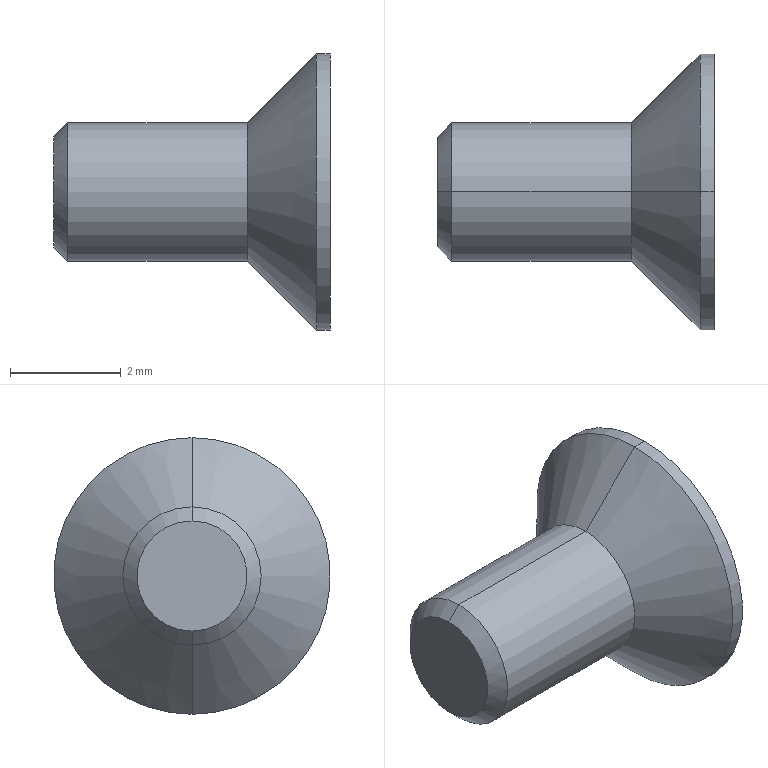Part | STEP file | 1 solid | 17 faces | box 5 x 5 x 5 mm | volume 34.882 mm3 | plane 9 | cylinder 4 | cone 4 | commonest cylinder face diameters 2.5 x2 5 x2
STEP:
#1=CARTESIAN_POINT('',(19.05,-14.605,5.12));
#2=VERTEX_POINT('',#1);
#3=CARTESIAN_POINT('',(19.05,-14.605,10.12));
#4=VERTEX_POINT('',#3);
#5=CARTESIAN_POINT('',(19.05,-14.605,7.62));
#6=DIRECTION('',(1.,0.,0.));
#7=DIRECTION('',(0.,0.,1.));
#8=AXIS2_PLACEMENT_3D('',#5,#6,#7);
#9=CIRCLE('',#8,2.5);
#10=EDGE_CURVE('',#2,#4,#9,.T.);
#11=ORIENTED_EDGE('',*,*,#10,.F.);
#12=CARTESIAN_POINT('',(18.8,-14.605,5.12));
#13=VERTEX_POINT('',#12);
#14=CARTESIAN_POINT('',(19.05,-14.605,5.12));
#15=DIRECTION('',(-1.,0.,0.));
#16=VECTOR('',#15,1000.);
#17=LINE('',#14,#16);
#18=EDGE_CURVE('',#2,#13,#17,.T.);
#19=ORIENTED_EDGE('',*,*,#18,.T.);
#20=CARTESIAN_POINT('',(18.8,-14.605,10.12));
#21=VERTEX_POINT('',#20);
#22=CARTESIAN_POINT('',(18.8,-14.605,7.62));
#23=DIRECTION('',(1.,0.,0.));
#24=DIRECTION('',(0.,0.,1.));
#25=AXIS2_PLACEMENT_3D('',#22,#23,#24);
#26=CIRCLE('',#25,2.5);
#27=EDGE_CURVE('',#13,#21,#26,.T.);
#28=ORIENTED_EDGE('',*,*,#27,.T.);
#29=CARTESIAN_POINT('',(19.05,-14.605,10.12));
#30=DIRECTION('',(-1.,0.,0.));
#31=VECTOR('',#30,1000.);
#32=LINE('',#29,#31);
#33=EDGE_CURVE('',#4,#21,#32,.T.);
#34=ORIENTED_EDGE('',*,*,#33,.F.);
#35=EDGE_LOOP('',(#11,#19,#28,#34));
#36=FACE_OUTER_BOUND('',#35,.T.);
#37=CARTESIAN_POINT('',(19.05,-14.605,7.62));
#38=DIRECTION('',(-1.,0.,0.));
#39=DIRECTION('',(0.,0.,1.));
#40=AXIS2_PLACEMENT_3D('',#37,#38,#39);
#41=CYLINDRICAL_SURFACE('',#40,2.5);
#42=ADVANCED_FACE('',(#36),#41,.T.);
#43=CARTESIAN_POINT('',(17.55,-14.605,6.37));
#44=VERTEX_POINT('',#43);
#45=CARTESIAN_POINT('',(17.55,-14.605,8.87));
#46=VERTEX_POINT('',#45);
#47=CARTESIAN_POINT('',(17.55,-14.605,7.62));
#48=DIRECTION('',(1.,0.,0.));
#49=DIRECTION('',(0.,0.,-1.));
#50=AXIS2_PLACEMENT_3D('',#47,#48,#49);
#51=CIRCLE('',#50,1.25);
#52=EDGE_CURVE('',#44,#46,#51,.T.);
#53=ORIENTED_EDGE('',*,*,#52,.T.);
#54=CARTESIAN_POINT('',(18.8,-14.605,10.12));
#55=DIRECTION('',(0.7071,0.,0.7071));
#56=VECTOR('',#55,1000.);
#57=LINE('',#54,#56);
#58=EDGE_CURVE('',#46,#21,#57,.T.);
#59=ORIENTED_EDGE('',*,*,#58,.T.);
#60=ORIENTED_EDGE('',*,*,#27,.F.);
#61=CARTESIAN_POINT('',(18.8,-14.605,5.12));
#62=DIRECTION('',(0.7071,0.,-0.7071));
#63=VECTOR('',#62,1000.);
#64=LINE('',#61,#63);
#65=EDGE_CURVE('',#44,#13,#64,.T.);
#66=ORIENTED_EDGE('',*,*,#65,.F.);
#67=EDGE_LOOP('',(#53,#59,#60,#66));
#68=FACE_OUTER_BOUND('',#67,.T.);
#69=CARTESIAN_POINT('',(18.8,-14.605,7.62));
#70=DIRECTION('',(1.,0.,0.));
#71=DIRECTION('',(0.,0.,-1.));
#72=AXIS2_PLACEMENT_3D('',#69,#70,#71);
#73=CONICAL_SURFACE('',#72,2.5,0.7854);
#74=ADVANCED_FACE('',(#68),#73,.T.);
#75=ORIENTED_EDGE('',*,*,#52,.F.);
#76=CARTESIAN_POINT('',(14.304,-14.605,6.37));
#77=VERTEX_POINT('',#76);
#78=CARTESIAN_POINT('',(19.05,-14.605,6.37));
#79=DIRECTION('',(-1.,0.,0.));
#80=VECTOR('',#79,1000.);
#81=LINE('',#78,#80);
#82=EDGE_CURVE('',#44,#77,#81,.T.);
#83=ORIENTED_EDGE('',*,*,#82,.T.);
#84=CARTESIAN_POINT('',(14.304,-14.605,8.87));
#85=VERTEX_POINT('',#84);
#86=CARTESIAN_POINT('',(14.304,-14.605,7.62));
#87=DIRECTION('',(1.,0.,0.));
#88=DIRECTION('',(0.,0.,1.));
#89=AXIS2_PLACEMENT_3D('',#86,#87,#88);
#90=CIRCLE('',#89,1.25);
#91=EDGE_CURVE('',#77,#85,#90,.T.);
#92=ORIENTED_EDGE('',*,*,#91,.T.);
#93=CARTESIAN_POINT('',(19.05,-14.605,8.87));
#94=DIRECTION('',(-1.,0.,0.));
#95=VECTOR('',#94,1000.);
#96=LINE('',#93,#95);
#97=EDGE_CURVE('',#46,#85,#96,.T.);
#98=ORIENTED_EDGE('',*,*,#97,.F.);
#99=EDGE_LOOP('',(#75,#83,#92,#98));
#100=FACE_OUTER_BOUND('',#99,.T.);
#101=CARTESIAN_POINT('',(19.05,-14.605,7.62));
#102=DIRECTION('',(-1.,0.,0.));
#103=DIRECTION('',(0.,0.,1.));
#104=AXIS2_PLACEMENT_3D('',#101,#102,#103);
#105=CYLINDRICAL_SURFACE('',#104,1.25);
#106=ADVANCED_FACE('',(#100),#105,.T.);
#107=CARTESIAN_POINT('',(14.05,-14.605,6.624));
#108=VERTEX_POINT('',#107);
#109=CARTESIAN_POINT('',(14.05,-14.605,8.616));
#110=VERTEX_POINT('',#109);
#111=CARTESIAN_POINT('',(14.05,-14.605,7.62));
#112=DIRECTION('',(1.,0.,0.));
#113=DIRECTION('',(0.,0.,-1.));
#114=AXIS2_PLACEMENT_3D('',#111,#112,#113);
#115=CIRCLE('',#114,0.996);
#116=EDGE_CURVE('',#108,#110,#115,.T.);
#117=ORIENTED_EDGE('',*,*,#116,.T.);
#118=CARTESIAN_POINT('',(14.304,-14.605,8.87));
#119=DIRECTION('',(0.7071,0.,0.7071));
#120=VECTOR('',#119,1000.);
#121=LINE('',#118,#120);
#122=EDGE_CURVE('',#110,#85,#121,.T.);
#123=ORIENTED_EDGE('',*,*,#122,.T.);
#124=ORIENTED_EDGE('',*,*,#91,.F.);
#125=CARTESIAN_POINT('',(14.304,-14.605,6.37));
#126=DIRECTION('',(0.7071,0.,-0.7071));
#127=VECTOR('',#126,1000.);
#128=LINE('',#125,#127);
#129=EDGE_CURVE('',#108,#77,#128,.T.);
#130=ORIENTED_EDGE('',*,*,#129,.F.);
#131=EDGE_LOOP('',(#117,#123,#124,#130));
#132=FACE_OUTER_BOUND('',#131,.T.);
#133=CARTESIAN_POINT('',(14.304,-14.605,7.62));
#134=DIRECTION('',(1.,0.,0.));
#135=DIRECTION('',(0.,0.,-1.));
#136=AXIS2_PLACEMENT_3D('',#133,#134,#135);
#137=CONICAL_SURFACE('',#136,1.25,0.7854);
#138=ADVANCED_FACE('',(#132),#137,.T.);
#139=CARTESIAN_POINT('',(19.05,-13.907,8.023));
#140=VERTEX_POINT('',#139);
#141=CARTESIAN_POINT('',(19.05,-13.907,7.217));
#142=VERTEX_POINT('',#141);
#143=CARTESIAN_POINT('',(19.05,-13.907,7.62));
#144=DIRECTION('',(0.,0.,-1.));
#145=VECTOR('',#144,1000.);
#146=LINE('',#143,#145);
#147=EDGE_CURVE('',#140,#142,#146,.T.);
#148=ORIENTED_EDGE('',*,*,#147,.T.);
#149=CARTESIAN_POINT('',(19.05,-14.605,6.813));
#150=VERTEX_POINT('',#149);
#151=CARTESIAN_POINT('',(19.05,-13.907,7.217));
#152=DIRECTION('',(0.,-0.866,-0.5));
#153=VECTOR('',#152,1000.);
#154=LINE('',#151,#153);
#155=EDGE_CURVE('',#142,#150,#154,.T.);
#156=ORIENTED_EDGE('',*,*,#155,.T.);
#157=CARTESIAN_POINT('',(19.05,-15.303,7.217));
#158=VERTEX_POINT('',#157);
#159=CARTESIAN_POINT('',(19.05,-14.605,6.813));
#160=DIRECTION('',(0.,-0.866,0.5));
#161=VECTOR('',#160,1000.);
#162=LINE('',#159,#161);
#163=EDGE_CURVE('',#150,#158,#162,.T.);
#164=ORIENTED_EDGE('',*,*,#163,.T.);
#165=CARTESIAN_POINT('',(19.05,-15.303,8.023));
#166=VERTEX_POINT('',#165);
#167=CARTESIAN_POINT('',(19.05,-15.303,7.62));
#168=DIRECTION('',(0.,0.,1.));
#169=VECTOR('',#168,1000.);
#170=LINE('',#167,#169);
#171=EDGE_CURVE('',#158,#166,#170,.T.);
#172=ORIENTED_EDGE('',*,*,#171,.T.);
#173=CARTESIAN_POINT('',(19.05,-14.605,8.427));
#174=VERTEX_POINT('',#173);
#175=CARTESIAN_POINT('',(19.05,-15.303,8.023));
#176=DIRECTION('',(0.,0.866,0.5));
#177=VECTOR('',#176,1000.);
#178=LINE('',#175,#177);
#179=EDGE_CURVE('',#166,#174,#178,.T.);
#180=ORIENTED_EDGE('',*,*,#179,.T.);
#181=CARTESIAN_POINT('',(19.05,-14.605,8.427));
#182=DIRECTION('',(0.,0.866,-0.5));
#183=VECTOR('',#182,1000.);
#184=LINE('',#181,#183);
#185=EDGE_CURVE('',#174,#140,#184,.T.);
#186=ORIENTED_EDGE('',*,*,#185,.T.);
#187=EDGE_LOOP('',(#148,#156,#164,#172,#180,#186));
#188=FACE_BOUND('',#187,.T.);
#189=CARTESIAN_POINT('',(19.05,-14.605,7.62));
#190=DIRECTION('',(1.,0.,0.));
#191=DIRECTION('',(0.,0.,1.));
#192=AXIS2_PLACEMENT_3D('',#189,#190,#191);
#193=CIRCLE('',#192,2.5);
#194=EDGE_CURVE('',#4,#2,#193,.T.);
#195=ORIENTED_EDGE('',*,*,#194,.T.);
#196=ORIENTED_EDGE('',*,*,#10,.T.);
#197=EDGE_LOOP('',(#195,#196));
#198=FACE_OUTER_BOUND('',#197,.T.);
#199=CARTESIAN_POINT('',(19.05,-12.105,7.62));
#200=DIRECTION('',(1.,0.,0.));
#201=DIRECTION('',(0.,1.,0.));
#202=AXIS2_PLACEMENT_3D('',#199,#200,#201);
#203=PLANE('',#202);
#204=ADVANCED_FACE('',(#188,#198),#203,.T.);
#205=ORIENTED_EDGE('',*,*,#18,.F.);
#206=ORIENTED_EDGE('',*,*,#194,.F.);
#207=ORIENTED_EDGE('',*,*,#33,.T.);
#208=CARTESIAN_POINT('',(18.8,-14.605,7.62));
#209=DIRECTION('',(1.,0.,0.));
#210=DIRECTION('',(0.,0.,1.));
#211=AXIS2_PLACEMENT_3D('',#208,#209,#210);
#212=CIRCLE('',#211,2.5);
#213=EDGE_CURVE('',#21,#13,#212,.T.);
#214=ORIENTED_EDGE('',*,*,#213,.T.);
#215=EDGE_LOOP('',(#205,#206,#207,#214));
#216=FACE_OUTER_BOUND('',#215,.T.);
#217=CARTESIAN_POINT('',(19.05,-14.605,7.62));
#218=DIRECTION('',(-1.,0.,0.));
#219=DIRECTION('',(0.,0.,1.));
#220=AXIS2_PLACEMENT_3D('',#217,#218,#219);
#221=CYLINDRICAL_SURFACE('',#220,2.5);
#222=ADVANCED_FACE('',(#216),#221,.T.);
#223=CARTESIAN_POINT('',(18.288,-13.907,7.217));
#224=VERTEX_POINT('',#223);
#225=CARTESIAN_POINT('',(18.288,-13.907,7.217));
#226=DIRECTION('',(1.,0.,0.));
#227=VECTOR('',#226,1000.);
#228=LINE('',#225,#227);
#229=EDGE_CURVE('',#224,#142,#228,.T.);
#230=ORIENTED_EDGE('',*,*,#229,.F.);
#231=CARTESIAN_POINT('',(18.288,-14.605,6.813));
#232=VERTEX_POINT('',#231);
#233=CARTESIAN_POINT('',(18.288,-14.605,6.813));
#234=DIRECTION('',(0.,0.866,0.5));
#235=VECTOR('',#234,1000.);
#236=LINE('',#233,#235);
#237=EDGE_CURVE('',#232,#224,#236,.T.);
#238=ORIENTED_EDGE('',*,*,#237,.F.);
#239=CARTESIAN_POINT('',(18.288,-14.605,6.813));
#240=DIRECTION('',(-1.,0.,0.));
#241=VECTOR('',#240,1000.);
#242=LINE('',#239,#241);
#243=EDGE_CURVE('',#150,#232,#242,.T.);
#244=ORIENTED_EDGE('',*,*,#243,.F.);
#245=ORIENTED_EDGE('',*,*,#155,.F.);
#246=EDGE_LOOP('',(#230,#238,#244,#245));
#247=FACE_OUTER_BOUND('',#246,.T.);
#248=CARTESIAN_POINT('',(18.288,-14.605,6.813));
#249=DIRECTION('',(0.,0.5,-0.866));
#250=DIRECTION('',(-1.,0.,0.));
#251=AXIS2_PLACEMENT_3D('',#248,#249,#250);
#252=PLANE('',#251);
#253=ADVANCED_FACE('',(#247),#252,.F.);
#254=CARTESIAN_POINT('',(18.288,-13.907,8.023));
#255=VERTEX_POINT('',#254);
#256=CARTESIAN_POINT('',(18.288,-13.907,8.023));
#257=DIRECTION('',(1.,0.,0.));
#258=VECTOR('',#257,1000.);
#259=LINE('',#256,#258);
#260=EDGE_CURVE('',#255,#140,#259,.T.);
#261=ORIENTED_EDGE('',*,*,#260,.F.);
#262=CARTESIAN_POINT('',(18.288,-13.907,7.217));
#263=DIRECTION('',(0.,0.,1.));
#264=VECTOR('',#263,1000.);
#265=LINE('',#262,#264);
#266=EDGE_CURVE('',#224,#255,#265,.T.);
#267=ORIENTED_EDGE('',*,*,#266,.F.);
#268=ORIENTED_EDGE('',*,*,#229,.T.);
#269=ORIENTED_EDGE('',*,*,#147,.F.);
#270=EDGE_LOOP('',(#261,#267,#268,#269));
#271=FACE_OUTER_BOUND('',#270,.T.);
#272=CARTESIAN_POINT('',(18.288,-13.907,7.217));
#273=DIRECTION('',(0.,1.,0.));
#274=DIRECTION('',(0.,0.,-1.));
#275=AXIS2_PLACEMENT_3D('',#272,#273,#274);
#276=PLANE('',#275);
#277=ADVANCED_FACE('',(#271),#276,.F.);
#278=CARTESIAN_POINT('',(18.288,-14.605,8.427));
#279=VERTEX_POINT('',#278);
#280=CARTESIAN_POINT('',(18.288,-14.605,8.427));
#281=DIRECTION('',(1.,0.,0.));
#282=VECTOR('',#281,1000.);
#283=LINE('',#280,#282);
#284=EDGE_CURVE('',#279,#174,#283,.T.);
#285=ORIENTED_EDGE('',*,*,#284,.F.);
#286=CARTESIAN_POINT('',(18.288,-13.907,8.023));
#287=DIRECTION('',(0.,-0.866,0.5));
#288=VECTOR('',#287,1000.);
#289=LINE('',#286,#288);
#290=EDGE_CURVE('',#255,#279,#289,.T.);
#291=ORIENTED_EDGE('',*,*,#290,.F.);
#292=ORIENTED_EDGE('',*,*,#260,.T.);
#293=ORIENTED_EDGE('',*,*,#185,.F.);
#294=EDGE_LOOP('',(#285,#291,#292,#293));
#295=FACE_OUTER_BOUND('',#294,.T.);
#296=CARTESIAN_POINT('',(18.288,-13.907,8.023));
#297=DIRECTION('',(0.,0.5,0.866));
#298=DIRECTION('',(1.,0.,0.));
#299=AXIS2_PLACEMENT_3D('',#296,#297,#298);
#300=PLANE('',#299);
#301=ADVANCED_FACE('',(#295),#300,.F.);
#302=CARTESIAN_POINT('',(18.288,-15.303,8.023));
#303=VERTEX_POINT('',#302);
#304=CARTESIAN_POINT('',(18.288,-15.303,8.023));
#305=DIRECTION('',(1.,0.,0.));
#306=VECTOR('',#305,1000.);
#307=LINE('',#304,#306);
#308=EDGE_CURVE('',#303,#166,#307,.T.);
#309=ORIENTED_EDGE('',*,*,#308,.F.);
#310=CARTESIAN_POINT('',(18.288,-14.605,8.427));
#311=DIRECTION('',(0.,-0.866,-0.5));
#312=VECTOR('',#311,1000.);
#313=LINE('',#310,#312);
#314=EDGE_CURVE('',#279,#303,#313,.T.);
#315=ORIENTED_EDGE('',*,*,#314,.F.);
#316=ORIENTED_EDGE('',*,*,#284,.T.);
#317=ORIENTED_EDGE('',*,*,#179,.F.);
#318=EDGE_LOOP('',(#309,#315,#316,#317));
#319=FACE_OUTER_BOUND('',#318,.T.);
#320=CARTESIAN_POINT('',(18.288,-14.605,8.427));
#321=DIRECTION('',(0.,-0.5,0.866));
#322=DIRECTION('',(-1.,0.,0.));
#323=AXIS2_PLACEMENT_3D('',#320,#321,#322);
#324=PLANE('',#323);
#325=ADVANCED_FACE('',(#319),#324,.F.);
#326=CARTESIAN_POINT('',(18.288,-15.303,7.217));
#327=VERTEX_POINT('',#326);
#328=CARTESIAN_POINT('',(18.288,-15.303,7.217));
#329=DIRECTION('',(1.,0.,0.));
#330=VECTOR('',#329,1000.);
#331=LINE('',#328,#330);
#332=EDGE_CURVE('',#327,#158,#331,.T.);
#333=ORIENTED_EDGE('',*,*,#332,.F.);
#334=CARTESIAN_POINT('',(18.288,-15.303,8.023));
#335=DIRECTION('',(0.,0.,-1.));
#336=VECTOR('',#335,1000.);
#337=LINE('',#334,#336);
#338=EDGE_CURVE('',#303,#327,#337,.T.);
#339=ORIENTED_EDGE('',*,*,#338,.F.);
#340=ORIENTED_EDGE('',*,*,#308,.T.);
#341=ORIENTED_EDGE('',*,*,#171,.F.);
#342=EDGE_LOOP('',(#333,#339,#340,#341));
#343=FACE_OUTER_BOUND('',#342,.T.);
#344=CARTESIAN_POINT('',(18.288,-15.303,8.023));
#345=DIRECTION('',(0.,-1.,0.));
#346=DIRECTION('',(0.,0.,-1.));
#347=AXIS2_PLACEMENT_3D('',#344,#345,#346);
#348=PLANE('',#347);
#349=ADVANCED_FACE('',(#343),#348,.F.);
#350=ORIENTED_EDGE('',*,*,#243,.T.);
#351=CARTESIAN_POINT('',(18.288,-15.303,7.217));
#352=DIRECTION('',(0.,0.866,-0.5));
#353=VECTOR('',#352,1000.);
#354=LINE('',#351,#353);
#355=EDGE_CURVE('',#327,#232,#354,.T.);
#356=ORIENTED_EDGE('',*,*,#355,.F.);
#357=ORIENTED_EDGE('',*,*,#332,.T.);
#358=ORIENTED_EDGE('',*,*,#163,.F.);
#359=EDGE_LOOP('',(#350,#356,#357,#358));
#360=FACE_OUTER_BOUND('',#359,.T.);
#361=CARTESIAN_POINT('',(18.288,-15.303,7.217));
#362=DIRECTION('',(0.,-0.5,-0.866));
#363=DIRECTION('',(0.,-0.866,0.5));
#364=AXIS2_PLACEMENT_3D('',#361,#362,#363);
#365=PLANE('',#364);
#366=ADVANCED_FACE('',(#360),#365,.F.);
#367=ORIENTED_EDGE('',*,*,#58,.F.);
#368=CARTESIAN_POINT('',(17.55,-14.605,7.62));
#369=DIRECTION('',(1.,0.,0.));
#370=DIRECTION('',(0.,0.,-1.));
#371=AXIS2_PLACEMENT_3D('',#368,#369,#370);
#372=CIRCLE('',#371,1.25);
#373=EDGE_CURVE('',#46,#44,#372,.T.);
#374=ORIENTED_EDGE('',*,*,#373,.T.);
#375=ORIENTED_EDGE('',*,*,#65,.T.);
#376=ORIENTED_EDGE('',*,*,#213,.F.);
#377=EDGE_LOOP('',(#367,#374,#375,#376));
#378=FACE_OUTER_BOUND('',#377,.T.);
#379=CARTESIAN_POINT('',(18.8,-14.605,7.62));
#380=DIRECTION('',(1.,0.,0.));
#381=DIRECTION('',(0.,0.,-1.));
#382=AXIS2_PLACEMENT_3D('',#379,#380,#381);
#383=CONICAL_SURFACE('',#382,2.5,0.7854);
#384=ADVANCED_FACE('',(#378),#383,.T.);
#385=ORIENTED_EDGE('',*,*,#314,.T.);
#386=ORIENTED_EDGE('',*,*,#338,.T.);
#387=ORIENTED_EDGE('',*,*,#355,.T.);
#388=ORIENTED_EDGE('',*,*,#237,.T.);
#389=ORIENTED_EDGE('',*,*,#266,.T.);
#390=ORIENTED_EDGE('',*,*,#290,.T.);
#391=EDGE_LOOP('',(#385,#386,#387,#388,#389,#390));
#392=FACE_OUTER_BOUND('',#391,.T.);
#393=CARTESIAN_POINT('',(18.288,0.,0.));
#394=DIRECTION('',(1.,0.,0.));
#395=DIRECTION('',(0.,1.,0.));
#396=AXIS2_PLACEMENT_3D('',#393,#394,#395);
#397=PLANE('',#396);
#398=ADVANCED_FACE('',(#392),#397,.T.);
#399=ORIENTED_EDGE('',*,*,#82,.F.);
#400=ORIENTED_EDGE('',*,*,#373,.F.);
#401=ORIENTED_EDGE('',*,*,#97,.T.);
#402=CARTESIAN_POINT('',(14.304,-14.605,7.62));
#403=DIRECTION('',(1.,0.,0.));
#404=DIRECTION('',(0.,0.,1.));
#405=AXIS2_PLACEMENT_3D('',#402,#403,#404);
#406=CIRCLE('',#405,1.25);
#407=EDGE_CURVE('',#85,#77,#406,.T.);
#408=ORIENTED_EDGE('',*,*,#407,.T.);
#409=EDGE_LOOP('',(#399,#400,#401,#408));
#410=FACE_OUTER_BOUND('',#409,.T.);
#411=CARTESIAN_POINT('',(19.05,-14.605,7.62));
#412=DIRECTION('',(-1.,0.,0.));
#413=DIRECTION('',(0.,0.,1.));
#414=AXIS2_PLACEMENT_3D('',#411,#412,#413);
#415=CYLINDRICAL_SURFACE('',#414,1.25);
#416=ADVANCED_FACE('',(#410),#415,.T.);
#417=ORIENTED_EDGE('',*,*,#122,.F.);
#418=CARTESIAN_POINT('',(14.05,-14.605,7.62));
#419=DIRECTION('',(1.,0.,0.));
#420=DIRECTION('',(0.,0.,-1.));
#421=AXIS2_PLACEMENT_3D('',#418,#419,#420);
#422=CIRCLE('',#421,0.996);
#423=EDGE_CURVE('',#110,#108,#422,.T.);
#424=ORIENTED_EDGE('',*,*,#423,.T.);
#425=ORIENTED_EDGE('',*,*,#129,.T.);
#426=ORIENTED_EDGE('',*,*,#407,.F.);
#427=EDGE_LOOP('',(#417,#424,#425,#426));
#428=FACE_OUTER_BOUND('',#427,.T.);
#429=CARTESIAN_POINT('',(14.304,-14.605,7.62));
#430=DIRECTION('',(1.,0.,0.));
#431=DIRECTION('',(0.,0.,-1.));
#432=AXIS2_PLACEMENT_3D('',#429,#430,#431);
#433=CONICAL_SURFACE('',#432,1.25,0.7854);
#434=ADVANCED_FACE('',(#428),#433,.T.);
#435=ORIENTED_EDGE('',*,*,#116,.F.);
#436=ORIENTED_EDGE('',*,*,#423,.F.);
#437=EDGE_LOOP('',(#435,#436));
#438=FACE_OUTER_BOUND('',#437,.T.);
#439=CARTESIAN_POINT('',(14.05,-14.605,7.62));
#440=DIRECTION('',(-1.,0.,0.));
#441=DIRECTION('',(0.,0.,1.));
#442=AXIS2_PLACEMENT_3D('',#439,#440,#441);
#443=PLANE('',#442);
#444=ADVANCED_FACE('',(#438),#443,.T.);
#445=CLOSED_SHELL('',(#42,#74,#106,#138,#204,#222,#253,#277,#301,#325,#349,#366,#384,#398,#416,#434,#444));
#446=MANIFOLD_SOLID_BREP('',#445);
#447=CARTESIAN_POINT('',(0.,0.,0.));
#448=DIRECTION('',(0.,0.,1.));
#449=DIRECTION('',(1.,0.,0.));
#450=AXIS2_PLACEMENT_3D('',#447,#448,#449);
#451=(LENGTH_UNIT()NAMED_UNIT(*)SI_UNIT(.MILLI.,.METRE.));
#452=UNCERTAINTY_MEASURE_WITH_UNIT(LENGTH_MEASURE(0.00001),#451,'','');
#453=(NAMED_UNIT(*)PLANE_ANGLE_UNIT()SI_UNIT($,.RADIAN.));
#454=(NAMED_UNIT(*)SI_UNIT($,.STERADIAN.)SOLID_ANGLE_UNIT());
#455=(GEOMETRIC_REPRESENTATION_CONTEXT(3)GLOBAL_UNCERTAINTY_ASSIGNED_CONTEXT((#452))GLOBAL_UNIT_ASSIGNED_CONTEXT((#451,#453,#454))REPRESENTATION_CONTEXT('',''));
#456=ADVANCED_BREP_SHAPE_REPRESENTATION('',(#446,#450),#455);